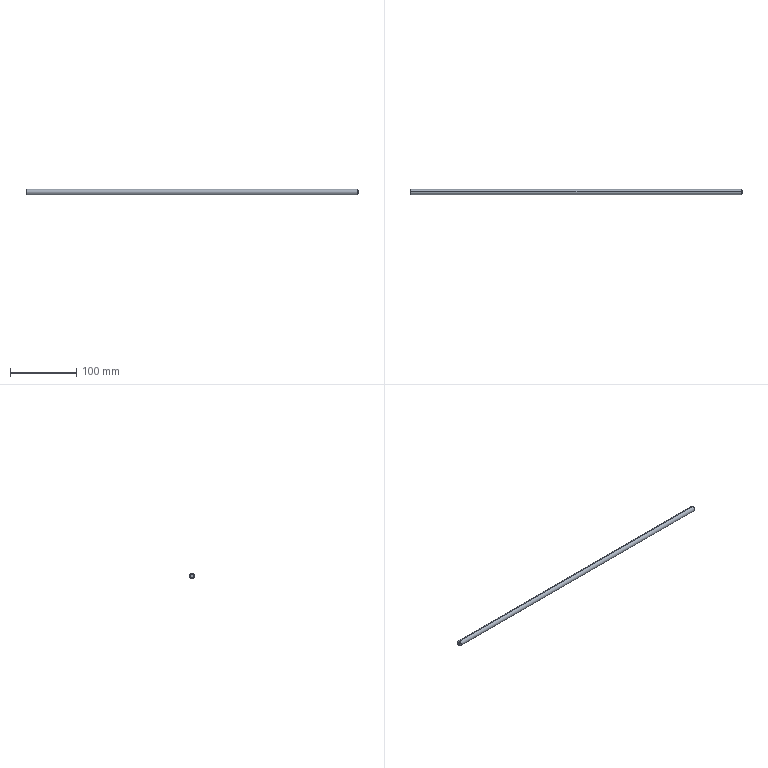Part | SolidWorks | features Chamfer 1, Extrusion 1 | 1 solid | 8 faces | box 500 x 8 x 8 mm | volume 25083 mm3 | cone 4 | cylinder 2 | plane 2 | commonest cylinder face diameters 8 x2
STEP:
#1=CARTESIAN_POINT('',(250.,0.,-2.5));
#2=VERTEX_POINT('',#1);
#3=CARTESIAN_POINT('',(250.,0.,2.5));
#4=VERTEX_POINT('',#3);
#5=CARTESIAN_POINT('',(250.,0.,0.));
#6=DIRECTION('',(1.,0.,0.));
#7=DIRECTION('',(0.,0.,-1.));
#8=AXIS2_PLACEMENT_3D('',#5,#6,#7);
#9=CIRCLE('',#8,2.5);
#10=EDGE_CURVE('',#2,#4,#9,.T.);
#11=ORIENTED_EDGE('',*,*,#10,.F.);
#12=CARTESIAN_POINT('',(248.5,0.,-4.));
#13=VERTEX_POINT('',#12);
#14=CARTESIAN_POINT('',(250.,0.,-2.5));
#15=DIRECTION('',(-0.7071,0.,-0.7071));
#16=VECTOR('',#15,1000.);
#17=LINE('',#14,#16);
#18=EDGE_CURVE('',#2,#13,#17,.T.);
#19=ORIENTED_EDGE('',*,*,#18,.T.);
#20=CARTESIAN_POINT('',(248.5,0.,4.));
#21=VERTEX_POINT('',#20);
#22=CARTESIAN_POINT('',(248.5,0.,0.));
#23=DIRECTION('',(-1.,0.,0.));
#24=DIRECTION('',(0.,0.,-1.));
#25=AXIS2_PLACEMENT_3D('',#22,#23,#24);
#26=CIRCLE('',#25,4.);
#27=EDGE_CURVE('',#21,#13,#26,.T.);
#28=ORIENTED_EDGE('',*,*,#27,.F.);
#29=CARTESIAN_POINT('',(250.,0.,2.5));
#30=DIRECTION('',(-0.7071,0.,0.7071));
#31=VECTOR('',#30,1000.);
#32=LINE('',#29,#31);
#33=EDGE_CURVE('',#4,#21,#32,.T.);
#34=ORIENTED_EDGE('',*,*,#33,.F.);
#35=EDGE_LOOP('',(#11,#19,#28,#34));
#36=FACE_OUTER_BOUND('',#35,.T.);
#37=CARTESIAN_POINT('',(250.,0.,0.));
#38=DIRECTION('',(-1.,0.,0.));
#39=DIRECTION('',(0.,0.,1.));
#40=AXIS2_PLACEMENT_3D('',#37,#38,#39);
#41=CONICAL_SURFACE('',#40,2.5,0.7854);
#42=ADVANCED_FACE('',(#36),#41,.T.);
#43=CARTESIAN_POINT('',(-250.,0.,2.5));
#44=VERTEX_POINT('',#43);
#45=CARTESIAN_POINT('',(-250.,0.,-2.5));
#46=VERTEX_POINT('',#45);
#47=CARTESIAN_POINT('',(-250.,0.,0.));
#48=DIRECTION('',(-1.,0.,0.));
#49=DIRECTION('',(0.,0.,-1.));
#50=AXIS2_PLACEMENT_3D('',#47,#48,#49);
#51=CIRCLE('',#50,2.5);
#52=EDGE_CURVE('',#44,#46,#51,.T.);
#53=ORIENTED_EDGE('',*,*,#52,.F.);
#54=CARTESIAN_POINT('',(-248.5,0.,4.));
#55=VERTEX_POINT('',#54);
#56=CARTESIAN_POINT('',(-248.5,0.,4.));
#57=DIRECTION('',(0.7071,0.,0.7071));
#58=VECTOR('',#57,1000.);
#59=LINE('',#56,#58);
#60=EDGE_CURVE('',#44,#55,#59,.T.);
#61=ORIENTED_EDGE('',*,*,#60,.T.);
#62=CARTESIAN_POINT('',(-248.5,0.,-4.));
#63=VERTEX_POINT('',#62);
#64=CARTESIAN_POINT('',(-248.5,0.,0.));
#65=DIRECTION('',(1.,0.,0.));
#66=DIRECTION('',(0.,0.,-1.));
#67=AXIS2_PLACEMENT_3D('',#64,#65,#66);
#68=CIRCLE('',#67,4.);
#69=EDGE_CURVE('',#63,#55,#68,.T.);
#70=ORIENTED_EDGE('',*,*,#69,.F.);
#71=CARTESIAN_POINT('',(-248.5,0.,-4.));
#72=DIRECTION('',(0.7071,0.,-0.7071));
#73=VECTOR('',#72,1000.);
#74=LINE('',#71,#73);
#75=EDGE_CURVE('',#46,#63,#74,.T.);
#76=ORIENTED_EDGE('',*,*,#75,.F.);
#77=EDGE_LOOP('',(#53,#61,#70,#76));
#78=FACE_OUTER_BOUND('',#77,.T.);
#79=CARTESIAN_POINT('',(-248.5,0.,0.));
#80=DIRECTION('',(1.,0.,0.));
#81=DIRECTION('',(0.,0.,-1.));
#82=AXIS2_PLACEMENT_3D('',#79,#80,#81);
#83=CONICAL_SURFACE('',#82,4.,0.7854);
#84=ADVANCED_FACE('',(#78),#83,.T.);
#85=ORIENTED_EDGE('',*,*,#27,.T.);
#86=CARTESIAN_POINT('',(250.,0.,-4.));
#87=DIRECTION('',(-1.,0.,0.));
#88=VECTOR('',#87,1000.);
#89=LINE('',#86,#88);
#90=EDGE_CURVE('',#13,#63,#89,.T.);
#91=ORIENTED_EDGE('',*,*,#90,.T.);
#92=ORIENTED_EDGE('',*,*,#69,.T.);
#93=CARTESIAN_POINT('',(250.,0.,4.));
#94=DIRECTION('',(-1.,0.,0.));
#95=VECTOR('',#94,1000.);
#96=LINE('',#93,#95);
#97=EDGE_CURVE('',#21,#55,#96,.T.);
#98=ORIENTED_EDGE('',*,*,#97,.F.);
#99=EDGE_LOOP('',(#85,#91,#92,#98));
#100=FACE_OUTER_BOUND('',#99,.T.);
#101=CARTESIAN_POINT('',(250.,0.,0.));
#102=DIRECTION('',(-1.,0.,0.));
#103=DIRECTION('',(0.,0.,1.));
#104=AXIS2_PLACEMENT_3D('',#101,#102,#103);
#105=CYLINDRICAL_SURFACE('',#104,4.);
#106=ADVANCED_FACE('',(#100),#105,.T.);
#107=ORIENTED_EDGE('',*,*,#90,.F.);
#108=CARTESIAN_POINT('',(248.5,0.,0.));
#109=DIRECTION('',(-1.,0.,0.));
#110=DIRECTION('',(0.,0.,-1.));
#111=AXIS2_PLACEMENT_3D('',#108,#109,#110);
#112=CIRCLE('',#111,4.);
#113=EDGE_CURVE('',#13,#21,#112,.T.);
#114=ORIENTED_EDGE('',*,*,#113,.T.);
#115=ORIENTED_EDGE('',*,*,#97,.T.);
#116=CARTESIAN_POINT('',(-248.5,0.,0.));
#117=DIRECTION('',(1.,0.,0.));
#118=DIRECTION('',(0.,0.,-1.));
#119=AXIS2_PLACEMENT_3D('',#116,#117,#118);
#120=CIRCLE('',#119,4.);
#121=EDGE_CURVE('',#55,#63,#120,.T.);
#122=ORIENTED_EDGE('',*,*,#121,.T.);
#123=EDGE_LOOP('',(#107,#114,#115,#122));
#124=FACE_OUTER_BOUND('',#123,.T.);
#125=CARTESIAN_POINT('',(250.,0.,0.));
#126=DIRECTION('',(-1.,0.,0.));
#127=DIRECTION('',(0.,0.,1.));
#128=AXIS2_PLACEMENT_3D('',#125,#126,#127);
#129=CYLINDRICAL_SURFACE('',#128,4.);
#130=ADVANCED_FACE('',(#124),#129,.T.);
#131=CARTESIAN_POINT('',(250.,0.,0.));
#132=DIRECTION('',(1.,0.,0.));
#133=DIRECTION('',(0.,0.,-1.));
#134=AXIS2_PLACEMENT_3D('',#131,#132,#133);
#135=CIRCLE('',#134,2.5);
#136=EDGE_CURVE('',#4,#2,#135,.T.);
#137=ORIENTED_EDGE('',*,*,#136,.T.);
#138=ORIENTED_EDGE('',*,*,#10,.T.);
#139=EDGE_LOOP('',(#137,#138));
#140=FACE_OUTER_BOUND('',#139,.T.);
#141=CARTESIAN_POINT('',(250.,0.,0.));
#142=DIRECTION('',(1.,0.,0.));
#143=DIRECTION('',(0.,0.,-1.));
#144=AXIS2_PLACEMENT_3D('',#141,#142,#143);
#145=PLANE('',#144);
#146=ADVANCED_FACE('',(#140),#145,.T.);
#147=CARTESIAN_POINT('',(-250.,0.,0.));
#148=DIRECTION('',(-1.,0.,0.));
#149=DIRECTION('',(0.,0.,-1.));
#150=AXIS2_PLACEMENT_3D('',#147,#148,#149);
#151=CIRCLE('',#150,2.5);
#152=EDGE_CURVE('',#46,#44,#151,.T.);
#153=ORIENTED_EDGE('',*,*,#152,.T.);
#154=ORIENTED_EDGE('',*,*,#52,.T.);
#155=EDGE_LOOP('',(#153,#154));
#156=FACE_OUTER_BOUND('',#155,.T.);
#157=CARTESIAN_POINT('',(-250.,0.,0.));
#158=DIRECTION('',(1.,0.,0.));
#159=DIRECTION('',(0.,0.,-1.));
#160=AXIS2_PLACEMENT_3D('',#157,#158,#159);
#161=PLANE('',#160);
#162=ADVANCED_FACE('',(#156),#161,.F.);
#163=ORIENTED_EDGE('',*,*,#60,.F.);
#164=ORIENTED_EDGE('',*,*,#152,.F.);
#165=ORIENTED_EDGE('',*,*,#75,.T.);
#166=ORIENTED_EDGE('',*,*,#121,.F.);
#167=EDGE_LOOP('',(#163,#164,#165,#166));
#168=FACE_OUTER_BOUND('',#167,.T.);
#169=CARTESIAN_POINT('',(-248.5,0.,0.));
#170=DIRECTION('',(1.,0.,0.));
#171=DIRECTION('',(0.,0.,-1.));
#172=AXIS2_PLACEMENT_3D('',#169,#170,#171);
#173=CONICAL_SURFACE('',#172,4.,0.7854);
#174=ADVANCED_FACE('',(#168),#173,.T.);
#175=ORIENTED_EDGE('',*,*,#18,.F.);
#176=ORIENTED_EDGE('',*,*,#136,.F.);
#177=ORIENTED_EDGE('',*,*,#33,.T.);
#178=ORIENTED_EDGE('',*,*,#113,.F.);
#179=EDGE_LOOP('',(#175,#176,#177,#178));
#180=FACE_OUTER_BOUND('',#179,.T.);
#181=CARTESIAN_POINT('',(250.,0.,0.));
#182=DIRECTION('',(-1.,0.,0.));
#183=DIRECTION('',(0.,0.,1.));
#184=AXIS2_PLACEMENT_3D('',#181,#182,#183);
#185=CONICAL_SURFACE('',#184,2.5,0.7854);
#186=ADVANCED_FACE('',(#180),#185,.T.);
#187=CLOSED_SHELL('',(#42,#84,#106,#130,#146,#162,#174,#186));
#188=MANIFOLD_SOLID_BREP('',#187);
#189=CARTESIAN_POINT('',(0.,0.,0.));
#190=DIRECTION('',(0.,0.,1.));
#191=DIRECTION('',(1.,0.,0.));
#192=AXIS2_PLACEMENT_3D('',#189,#190,#191);
#193=(LENGTH_UNIT()NAMED_UNIT(*)SI_UNIT(.MILLI.,.METRE.));
#194=UNCERTAINTY_MEASURE_WITH_UNIT(LENGTH_MEASURE(0.00001),#193,'','');
#195=(NAMED_UNIT(*)PLANE_ANGLE_UNIT()SI_UNIT($,.RADIAN.));
#196=(NAMED_UNIT(*)SI_UNIT($,.STERADIAN.)SOLID_ANGLE_UNIT());
#197=(GEOMETRIC_REPRESENTATION_CONTEXT(3)GLOBAL_UNCERTAINTY_ASSIGNED_CONTEXT((#194))GLOBAL_UNIT_ASSIGNED_CONTEXT((#193,#195,#196))REPRESENTATION_CONTEXT('',''));
#198=ADVANCED_BREP_SHAPE_REPRESENTATION('',(#188,#192),#197);